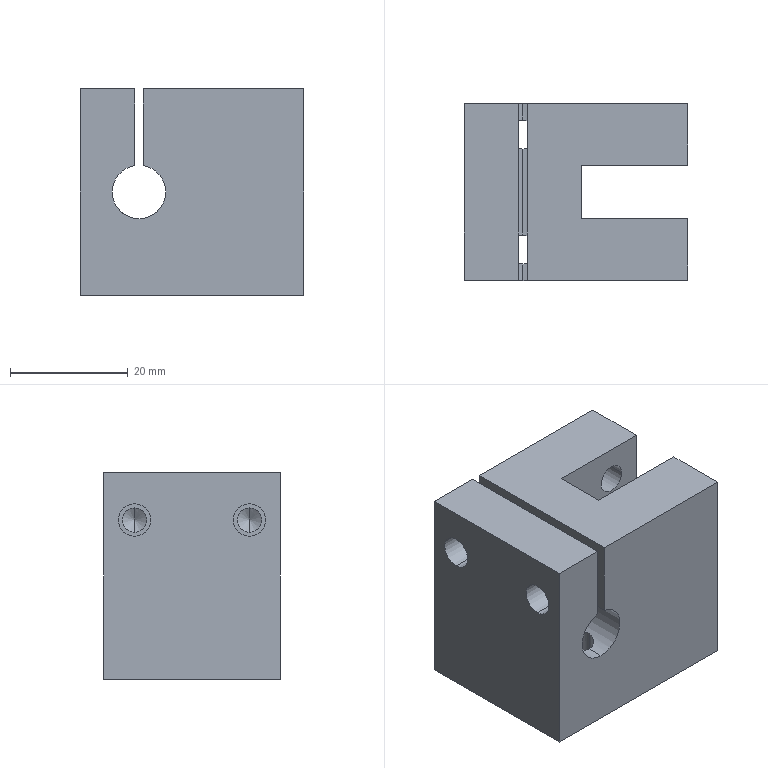Part | STEP file | DCV-000-020 | 1 solid | 35 faces | box 38 x 30 x 35 mm | volume 29966 mm3 | cylinder 18 | plane 13 | cone 4 | commonest cylinder face diameters 4.917 x8 4.134 x4 5.5 x4 9.1 x2